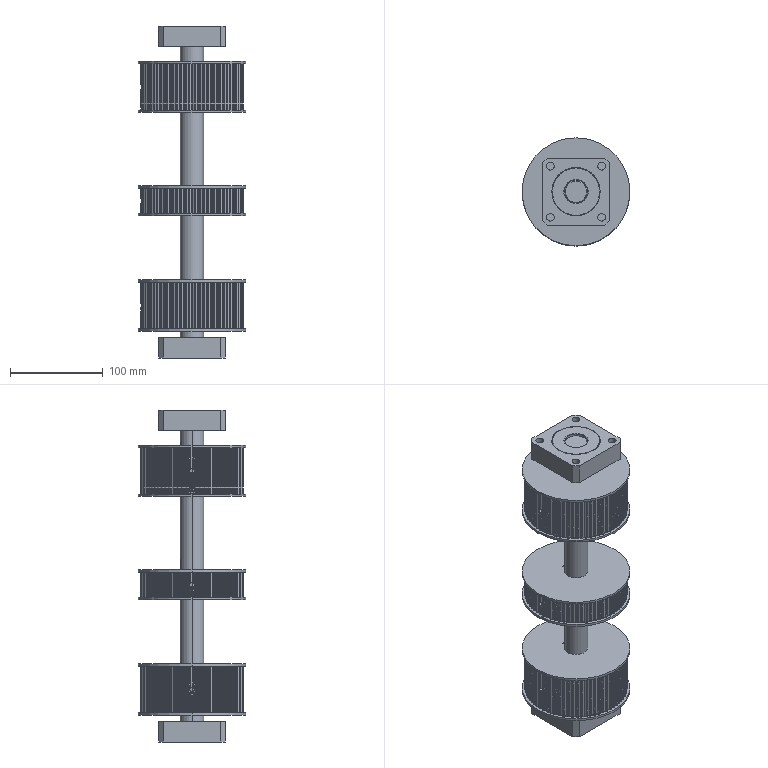Part | 8 solids | 1171 faces | box 116 x 116 x 357 mm | volume 1597800 mm3 | cylinder 1081 | plane 70 | cone 20 | commonest cylinder face diameters 2.5 x771 110 x219 8.5 x16 13 x16 25 x15 0.6 x12